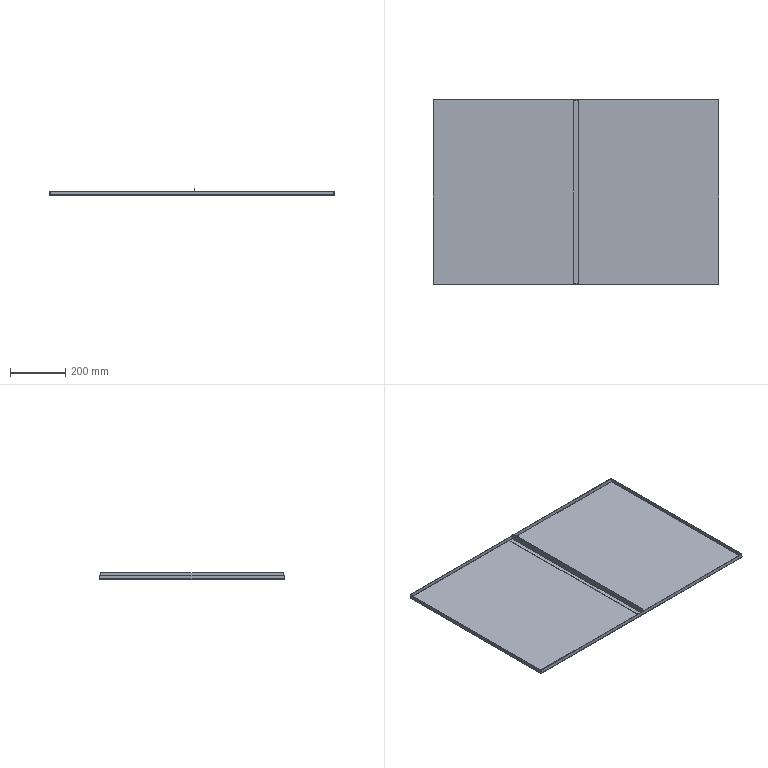Part | SolidWorks | 2 solids | 52 faces | box 1030 x 670 x 23.5 mm | volume 1500573 mm3 | plane 34 | cylinder 10 | spline 8 | commonest cylinder face diameters 0.2 x5 4.2 x4 3.2 x1